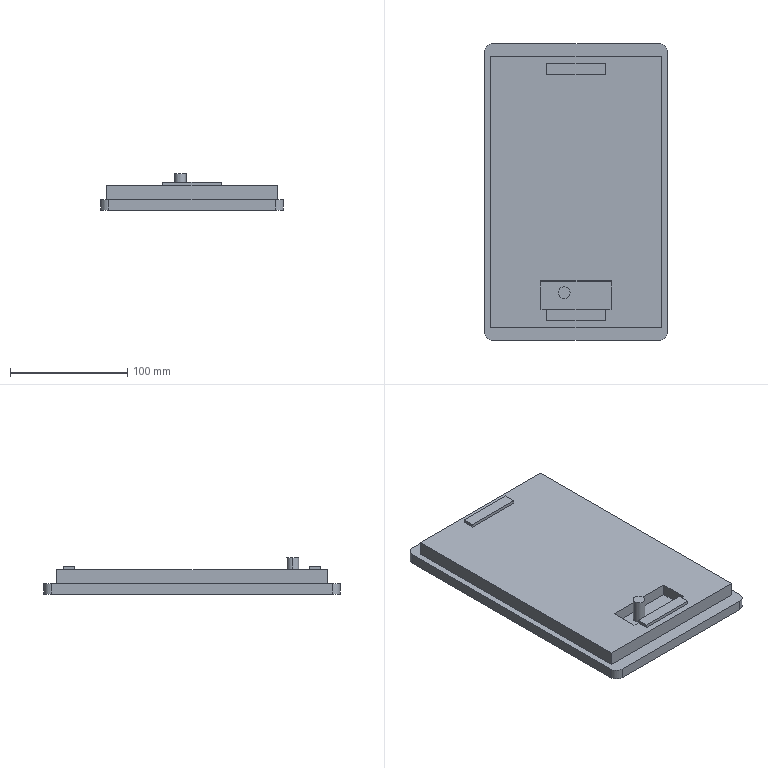Part | 1 solid | 37 faces | box 156 x 253.2 x 31 mm | volume 746157 mm3 | plane 31 | cylinder 6 | commonest cylinder face diameters 14 x4 10 x2
STEP:
#1=CARTESIAN_POINT('',(-5.,-86.,31.));
#2=VERTEX_POINT('',#1);
#3=CARTESIAN_POINT('',(-15.,-86.,31.));
#4=VERTEX_POINT('',#3);
#5=CARTESIAN_POINT('',(-10.,-86.,31.));
#6=DIRECTION('',(0.,0.,1.));
#7=DIRECTION('',(1.,0.,0.));
#8=AXIS2_PLACEMENT_3D('',#5,#6,#7);
#9=CIRCLE('',#8,5.);
#10=EDGE_CURVE('',#2,#4,#9,.T.);
#11=ORIENTED_EDGE('',*,*,#10,.F.);
#12=CARTESIAN_POINT('',(-5.,-86.,11.));
#13=VERTEX_POINT('',#12);
#14=CARTESIAN_POINT('',(-5.,-86.,31.));
#15=DIRECTION('',(0.,0.,-1.));
#16=VECTOR('',#15,1000.);
#17=LINE('',#14,#16);
#18=EDGE_CURVE('',#2,#13,#17,.T.);
#19=ORIENTED_EDGE('',*,*,#18,.T.);
#20=CARTESIAN_POINT('',(-15.,-86.,11.));
#21=VERTEX_POINT('',#20);
#22=CARTESIAN_POINT('',(-10.,-86.,11.));
#23=DIRECTION('',(0.,0.,1.));
#24=DIRECTION('',(1.,0.,0.));
#25=AXIS2_PLACEMENT_3D('',#22,#23,#24);
#26=CIRCLE('',#25,5.);
#27=EDGE_CURVE('',#13,#21,#26,.T.);
#28=ORIENTED_EDGE('',*,*,#27,.T.);
#29=CARTESIAN_POINT('',(-15.,-86.,31.));
#30=DIRECTION('',(0.,0.,-1.));
#31=VECTOR('',#30,1000.);
#32=LINE('',#29,#31);
#33=EDGE_CURVE('',#4,#21,#32,.T.);
#34=ORIENTED_EDGE('',*,*,#33,.F.);
#35=EDGE_LOOP('',(#11,#19,#28,#34));
#36=FACE_OUTER_BOUND('',#35,.T.);
#37=CARTESIAN_POINT('',(-10.,-86.,31.));
#38=DIRECTION('',(0.,0.,-1.));
#39=DIRECTION('',(-1.,0.,0.));
#40=AXIS2_PLACEMENT_3D('',#37,#38,#39);
#41=CYLINDRICAL_SURFACE('',#40,5.);
#42=ADVANCED_FACE('',(#36),#41,.T.);
#43=CARTESIAN_POINT('',(25.,-100.,21.));
#44=VERTEX_POINT('',#43);
#45=CARTESIAN_POINT('',(30.,-100.,21.));
#46=VERTEX_POINT('',#45);
#47=CARTESIAN_POINT('',(-30.,-100.,21.));
#48=DIRECTION('',(1.,0.,0.));
#49=VECTOR('',#48,1000.);
#50=LINE('',#47,#49);
#51=EDGE_CURVE('',#44,#46,#50,.T.);
#52=ORIENTED_EDGE('',*,*,#51,.F.);
#53=CARTESIAN_POINT('',(25.,-110.,21.));
#54=VERTEX_POINT('',#53);
#55=CARTESIAN_POINT('',(25.,-110.,21.));
#56=DIRECTION('',(0.,1.,0.));
#57=VECTOR('',#56,1000.);
#58=LINE('',#55,#57);
#59=EDGE_CURVE('',#54,#44,#58,.T.);
#60=ORIENTED_EDGE('',*,*,#59,.F.);
#61=CARTESIAN_POINT('',(-25.,-110.,21.));
#62=VERTEX_POINT('',#61);
#63=CARTESIAN_POINT('',(-25.,-110.,21.));
#64=DIRECTION('',(1.,0.,0.));
#65=VECTOR('',#64,1000.);
#66=LINE('',#63,#65);
#67=EDGE_CURVE('',#62,#54,#66,.T.);
#68=ORIENTED_EDGE('',*,*,#67,.F.);
#69=CARTESIAN_POINT('',(-25.,-100.,21.));
#70=VERTEX_POINT('',#69);
#71=CARTESIAN_POINT('',(-25.,-110.,21.));
#72=DIRECTION('',(0.,-1.,0.));
#73=VECTOR('',#72,1000.);
#74=LINE('',#71,#73);
#75=EDGE_CURVE('',#70,#62,#74,.T.);
#76=ORIENTED_EDGE('',*,*,#75,.F.);
#77=CARTESIAN_POINT('',(-30.,-100.,21.));
#78=VERTEX_POINT('',#77);
#79=CARTESIAN_POINT('',(-30.,-100.,21.));
#80=DIRECTION('',(1.,0.,0.));
#81=VECTOR('',#80,1000.);
#82=LINE('',#79,#81);
#83=EDGE_CURVE('',#78,#70,#82,.T.);
#84=ORIENTED_EDGE('',*,*,#83,.F.);
#85=CARTESIAN_POINT('',(-30.,-76.,21.));
#86=VERTEX_POINT('',#85);
#87=CARTESIAN_POINT('',(-30.,-76.,21.));
#88=DIRECTION('',(0.,-1.,0.));
#89=VECTOR('',#88,1000.);
#90=LINE('',#87,#89);
#91=EDGE_CURVE('',#86,#78,#90,.T.);
#92=ORIENTED_EDGE('',*,*,#91,.F.);
#93=CARTESIAN_POINT('',(30.,-76.,21.));
#94=VERTEX_POINT('',#93);
#95=CARTESIAN_POINT('',(-30.,-76.,21.));
#96=DIRECTION('',(-1.,0.,0.));
#97=VECTOR('',#96,1000.);
#98=LINE('',#95,#97);
#99=EDGE_CURVE('',#94,#86,#98,.T.);
#100=ORIENTED_EDGE('',*,*,#99,.F.);
#101=CARTESIAN_POINT('',(30.,-76.,21.));
#102=DIRECTION('',(0.,1.,0.));
#103=VECTOR('',#102,1000.);
#104=LINE('',#101,#103);
#105=EDGE_CURVE('',#46,#94,#104,.T.);
#106=ORIENTED_EDGE('',*,*,#105,.F.);
#107=EDGE_LOOP('',(#52,#60,#68,#76,#84,#92,#100,#106));
#108=FACE_BOUND('',#107,.T.);
#109=CARTESIAN_POINT('',(72.75,-115.5,21.));
#110=VERTEX_POINT('',#109);
#111=CARTESIAN_POINT('',(72.75,115.5,21.));
#112=VERTEX_POINT('',#111);
#113=CARTESIAN_POINT('',(72.75,115.5,21.));
#114=DIRECTION('',(0.,1.,0.));
#115=VECTOR('',#114,1000.);
#116=LINE('',#113,#115);
#117=EDGE_CURVE('',#110,#112,#116,.T.);
#118=ORIENTED_EDGE('',*,*,#117,.T.);
#119=CARTESIAN_POINT('',(-72.75,115.5,21.));
#120=VERTEX_POINT('',#119);
#121=CARTESIAN_POINT('',(-72.75,115.5,21.));
#122=DIRECTION('',(-1.,0.,0.));
#123=VECTOR('',#122,1000.);
#124=LINE('',#121,#123);
#125=EDGE_CURVE('',#112,#120,#124,.T.);
#126=ORIENTED_EDGE('',*,*,#125,.T.);
#127=CARTESIAN_POINT('',(-72.75,-115.5,21.));
#128=VERTEX_POINT('',#127);
#129=CARTESIAN_POINT('',(-72.75,115.5,21.));
#130=DIRECTION('',(0.,-1.,0.));
#131=VECTOR('',#130,1000.);
#132=LINE('',#129,#131);
#133=EDGE_CURVE('',#120,#128,#132,.T.);
#134=ORIENTED_EDGE('',*,*,#133,.T.);
#135=CARTESIAN_POINT('',(-72.75,-115.5,21.));
#136=DIRECTION('',(1.,0.,0.));
#137=VECTOR('',#136,1000.);
#138=LINE('',#135,#137);
#139=EDGE_CURVE('',#128,#110,#138,.T.);
#140=ORIENTED_EDGE('',*,*,#139,.T.);
#141=EDGE_LOOP('',(#118,#126,#134,#140));
#142=FACE_OUTER_BOUND('',#141,.T.);
#143=CARTESIAN_POINT('',(25.,110.,21.));
#144=VERTEX_POINT('',#143);
#145=CARTESIAN_POINT('',(-25.,110.,21.));
#146=VERTEX_POINT('',#145);
#147=CARTESIAN_POINT('',(-25.,110.,21.));
#148=DIRECTION('',(-1.,0.,0.));
#149=VECTOR('',#148,1000.);
#150=LINE('',#147,#149);
#151=EDGE_CURVE('',#144,#146,#150,.T.);
#152=ORIENTED_EDGE('',*,*,#151,.F.);
#153=CARTESIAN_POINT('',(25.,100.,21.));
#154=VERTEX_POINT('',#153);
#155=CARTESIAN_POINT('',(25.,110.,21.));
#156=DIRECTION('',(0.,1.,0.));
#157=VECTOR('',#156,1000.);
#158=LINE('',#155,#157);
#159=EDGE_CURVE('',#154,#144,#158,.T.);
#160=ORIENTED_EDGE('',*,*,#159,.F.);
#161=CARTESIAN_POINT('',(-25.,100.,21.));
#162=VERTEX_POINT('',#161);
#163=CARTESIAN_POINT('',(-25.,100.,21.));
#164=DIRECTION('',(1.,0.,0.));
#165=VECTOR('',#164,1000.);
#166=LINE('',#163,#165);
#167=EDGE_CURVE('',#162,#154,#166,.T.);
#168=ORIENTED_EDGE('',*,*,#167,.F.);
#169=CARTESIAN_POINT('',(-25.,110.,21.));
#170=DIRECTION('',(0.,-1.,0.));
#171=VECTOR('',#170,1000.);
#172=LINE('',#169,#171);
#173=EDGE_CURVE('',#146,#162,#172,.T.);
#174=ORIENTED_EDGE('',*,*,#173,.F.);
#175=EDGE_LOOP('',(#152,#160,#168,#174));
#176=FACE_BOUND('',#175,.T.);
#177=CARTESIAN_POINT('',(0.,0.,21.));
#178=DIRECTION('',(0.,0.,1.));
#179=DIRECTION('',(1.,0.,0.));
#180=AXIS2_PLACEMENT_3D('',#177,#178,#179);
#181=PLANE('',#180);
#182=ADVANCED_FACE('',(#108,#142,#176),#181,.T.);
#183=CARTESIAN_POINT('',(78.,-119.6,9.));
#184=VERTEX_POINT('',#183);
#185=CARTESIAN_POINT('',(78.,119.6,9.));
#186=VERTEX_POINT('',#185);
#187=CARTESIAN_POINT('',(78.,126.6,9.));
#188=DIRECTION('',(0.,1.,0.));
#189=VECTOR('',#188,1000.);
#190=LINE('',#187,#189);
#191=EDGE_CURVE('',#184,#186,#190,.T.);
#192=ORIENTED_EDGE('',*,*,#191,.F.);
#193=CARTESIAN_POINT('',(78.,-119.6,0.));
#194=VERTEX_POINT('',#193);
#195=CARTESIAN_POINT('',(78.,-119.6,9.));
#196=DIRECTION('',(0.,0.,-1.));
#197=VECTOR('',#196,1000.);
#198=LINE('',#195,#197);
#199=EDGE_CURVE('',#184,#194,#198,.T.);
#200=ORIENTED_EDGE('',*,*,#199,.T.);
#201=CARTESIAN_POINT('',(78.,119.6,0.));
#202=VERTEX_POINT('',#201);
#203=CARTESIAN_POINT('',(78.,126.6,0.));
#204=DIRECTION('',(0.,1.,0.));
#205=VECTOR('',#204,1000.);
#206=LINE('',#203,#205);
#207=EDGE_CURVE('',#194,#202,#206,.T.);
#208=ORIENTED_EDGE('',*,*,#207,.T.);
#209=CARTESIAN_POINT('',(78.,119.6,9.));
#210=DIRECTION('',(0.,0.,1.));
#211=VECTOR('',#210,1000.);
#212=LINE('',#209,#211);
#213=EDGE_CURVE('',#202,#186,#212,.T.);
#214=ORIENTED_EDGE('',*,*,#213,.T.);
#215=EDGE_LOOP('',(#192,#200,#208,#214));
#216=FACE_OUTER_BOUND('',#215,.T.);
#217=CARTESIAN_POINT('',(78.,126.6,9.));
#218=DIRECTION('',(-1.,0.,0.));
#219=DIRECTION('',(0.,-1.,0.));
#220=AXIS2_PLACEMENT_3D('',#217,#218,#219);
#221=PLANE('',#220);
#222=ADVANCED_FACE('',(#216),#221,.F.);
#223=CARTESIAN_POINT('',(71.,126.6,9.));
#224=VERTEX_POINT('',#223);
#225=CARTESIAN_POINT('',(-71.,126.6,9.));
#226=VERTEX_POINT('',#225);
#227=CARTESIAN_POINT('',(-78.,126.6,9.));
#228=DIRECTION('',(-1.,0.,0.));
#229=VECTOR('',#228,1000.);
#230=LINE('',#227,#229);
#231=EDGE_CURVE('',#224,#226,#230,.T.);
#232=ORIENTED_EDGE('',*,*,#231,.F.);
#233=CARTESIAN_POINT('',(71.,126.6,0.));
#234=VERTEX_POINT('',#233);
#235=CARTESIAN_POINT('',(71.,126.6,9.));
#236=DIRECTION('',(0.,0.,-1.));
#237=VECTOR('',#236,1000.);
#238=LINE('',#235,#237);
#239=EDGE_CURVE('',#224,#234,#238,.T.);
#240=ORIENTED_EDGE('',*,*,#239,.T.);
#241=CARTESIAN_POINT('',(-71.,126.6,0.));
#242=VERTEX_POINT('',#241);
#243=CARTESIAN_POINT('',(-78.,126.6,0.));
#244=DIRECTION('',(-1.,0.,0.));
#245=VECTOR('',#244,1000.);
#246=LINE('',#243,#245);
#247=EDGE_CURVE('',#234,#242,#246,.T.);
#248=ORIENTED_EDGE('',*,*,#247,.T.);
#249=CARTESIAN_POINT('',(-71.,126.6,9.));
#250=DIRECTION('',(0.,0.,1.));
#251=VECTOR('',#250,1000.);
#252=LINE('',#249,#251);
#253=EDGE_CURVE('',#242,#226,#252,.T.);
#254=ORIENTED_EDGE('',*,*,#253,.T.);
#255=EDGE_LOOP('',(#232,#240,#248,#254));
#256=FACE_OUTER_BOUND('',#255,.T.);
#257=CARTESIAN_POINT('',(-78.,126.6,9.));
#258=DIRECTION('',(0.,-1.,0.));
#259=DIRECTION('',(0.,0.,-1.));
#260=AXIS2_PLACEMENT_3D('',#257,#258,#259);
#261=PLANE('',#260);
#262=ADVANCED_FACE('',(#256),#261,.F.);
#263=CARTESIAN_POINT('',(-78.,119.6,0.));
#264=VERTEX_POINT('',#263);
#265=CARTESIAN_POINT('',(-78.,-119.6,0.));
#266=VERTEX_POINT('',#265);
#267=CARTESIAN_POINT('',(-78.,126.6,0.));
#268=DIRECTION('',(0.,-1.,0.));
#269=VECTOR('',#268,1000.);
#270=LINE('',#267,#269);
#271=EDGE_CURVE('',#264,#266,#270,.T.);
#272=ORIENTED_EDGE('',*,*,#271,.T.);
#273=CARTESIAN_POINT('',(-78.,-119.6,9.));
#274=VERTEX_POINT('',#273);
#275=CARTESIAN_POINT('',(-78.,-119.6,9.));
#276=DIRECTION('',(0.,0.,1.));
#277=VECTOR('',#276,1000.);
#278=LINE('',#275,#277);
#279=EDGE_CURVE('',#266,#274,#278,.T.);
#280=ORIENTED_EDGE('',*,*,#279,.T.);
#281=CARTESIAN_POINT('',(-78.,119.6,9.));
#282=VERTEX_POINT('',#281);
#283=CARTESIAN_POINT('',(-78.,126.6,9.));
#284=DIRECTION('',(0.,-1.,0.));
#285=VECTOR('',#284,1000.);
#286=LINE('',#283,#285);
#287=EDGE_CURVE('',#282,#274,#286,.T.);
#288=ORIENTED_EDGE('',*,*,#287,.F.);
#289=CARTESIAN_POINT('',(-78.,119.6,9.));
#290=DIRECTION('',(0.,0.,-1.));
#291=VECTOR('',#290,1000.);
#292=LINE('',#289,#291);
#293=EDGE_CURVE('',#282,#264,#292,.T.);
#294=ORIENTED_EDGE('',*,*,#293,.T.);
#295=EDGE_LOOP('',(#272,#280,#288,#294));
#296=FACE_OUTER_BOUND('',#295,.T.);
#297=CARTESIAN_POINT('',(-78.,126.6,9.));
#298=DIRECTION('',(1.,0.,0.));
#299=DIRECTION('',(0.,1.,0.));
#300=AXIS2_PLACEMENT_3D('',#297,#298,#299);
#301=PLANE('',#300);
#302=ADVANCED_FACE('',(#296),#301,.F.);
#303=CARTESIAN_POINT('',(-71.,-126.6,0.));
#304=VERTEX_POINT('',#303);
#305=CARTESIAN_POINT('',(71.,-126.6,0.));
#306=VERTEX_POINT('',#305);
#307=CARTESIAN_POINT('',(-78.,-126.6,0.));
#308=DIRECTION('',(1.,0.,0.));
#309=VECTOR('',#308,1000.);
#310=LINE('',#307,#309);
#311=EDGE_CURVE('',#304,#306,#310,.T.);
#312=ORIENTED_EDGE('',*,*,#311,.T.);
#313=CARTESIAN_POINT('',(71.,-126.6,9.));
#314=VERTEX_POINT('',#313);
#315=CARTESIAN_POINT('',(71.,-126.6,9.));
#316=DIRECTION('',(0.,0.,1.));
#317=VECTOR('',#316,1000.);
#318=LINE('',#315,#317);
#319=EDGE_CURVE('',#306,#314,#318,.T.);
#320=ORIENTED_EDGE('',*,*,#319,.T.);
#321=CARTESIAN_POINT('',(-71.,-126.6,9.));
#322=VERTEX_POINT('',#321);
#323=CARTESIAN_POINT('',(-78.,-126.6,9.));
#324=DIRECTION('',(1.,0.,0.));
#325=VECTOR('',#324,1000.);
#326=LINE('',#323,#325);
#327=EDGE_CURVE('',#322,#314,#326,.T.);
#328=ORIENTED_EDGE('',*,*,#327,.F.);
#329=CARTESIAN_POINT('',(-71.,-126.6,9.));
#330=DIRECTION('',(0.,0.,-1.));
#331=VECTOR('',#330,1000.);
#332=LINE('',#329,#331);
#333=EDGE_CURVE('',#322,#304,#332,.T.);
#334=ORIENTED_EDGE('',*,*,#333,.T.);
#335=EDGE_LOOP('',(#312,#320,#328,#334));
#336=FACE_OUTER_BOUND('',#335,.T.);
#337=CARTESIAN_POINT('',(-78.,-126.6,9.));
#338=DIRECTION('',(0.,1.,0.));
#339=DIRECTION('',(0.,0.,1.));
#340=AXIS2_PLACEMENT_3D('',#337,#338,#339);
#341=PLANE('',#340);
#342=ADVANCED_FACE('',(#336),#341,.F.);
#343=CARTESIAN_POINT('',(72.75,-115.5,9.));
#344=VERTEX_POINT('',#343);
#345=CARTESIAN_POINT('',(72.75,115.5,9.));
#346=VERTEX_POINT('',#345);
#347=CARTESIAN_POINT('',(72.75,115.5,9.));
#348=DIRECTION('',(0.,1.,0.));
#349=VECTOR('',#348,1000.);
#350=LINE('',#347,#349);
#351=EDGE_CURVE('',#344,#346,#350,.T.);
#352=ORIENTED_EDGE('',*,*,#351,.F.);
#353=CARTESIAN_POINT('',(-72.75,-115.5,9.));
#354=VERTEX_POINT('',#353);
#355=CARTESIAN_POINT('',(-72.75,-115.5,9.));
#356=DIRECTION('',(1.,0.,0.));
#357=VECTOR('',#356,1000.);
#358=LINE('',#355,#357);
#359=EDGE_CURVE('',#354,#344,#358,.T.);
#360=ORIENTED_EDGE('',*,*,#359,.F.);
#361=CARTESIAN_POINT('',(-72.75,115.5,9.));
#362=VERTEX_POINT('',#361);
#363=CARTESIAN_POINT('',(-72.75,115.5,9.));
#364=DIRECTION('',(0.,-1.,0.));
#365=VECTOR('',#364,1000.);
#366=LINE('',#363,#365);
#367=EDGE_CURVE('',#362,#354,#366,.T.);
#368=ORIENTED_EDGE('',*,*,#367,.F.);
#369=CARTESIAN_POINT('',(-72.75,115.5,9.));
#370=DIRECTION('',(-1.,0.,0.));
#371=VECTOR('',#370,1000.);
#372=LINE('',#369,#371);
#373=EDGE_CURVE('',#346,#362,#372,.T.);
#374=ORIENTED_EDGE('',*,*,#373,.F.);
#375=EDGE_LOOP('',(#352,#360,#368,#374));
#376=FACE_BOUND('',#375,.T.);
#377=ORIENTED_EDGE('',*,*,#327,.T.);
#378=CARTESIAN_POINT('',(71.,-119.6,9.));
#379=DIRECTION('',(0.,0.,1.));
#380=DIRECTION('',(1.,0.,0.));
#381=AXIS2_PLACEMENT_3D('',#378,#379,#380);
#382=CIRCLE('',#381,7.);
#383=EDGE_CURVE('',#314,#184,#382,.T.);
#384=ORIENTED_EDGE('',*,*,#383,.T.);
#385=ORIENTED_EDGE('',*,*,#191,.T.);
#386=CARTESIAN_POINT('',(71.,119.6,9.));
#387=DIRECTION('',(0.,0.,1.));
#388=DIRECTION('',(1.,0.,0.));
#389=AXIS2_PLACEMENT_3D('',#386,#387,#388);
#390=CIRCLE('',#389,7.);
#391=EDGE_CURVE('',#186,#224,#390,.T.);
#392=ORIENTED_EDGE('',*,*,#391,.T.);
#393=ORIENTED_EDGE('',*,*,#231,.T.);
#394=CARTESIAN_POINT('',(-71.,119.6,9.));
#395=DIRECTION('',(0.,0.,1.));
#396=DIRECTION('',(1.,0.,0.));
#397=AXIS2_PLACEMENT_3D('',#394,#395,#396);
#398=CIRCLE('',#397,7.);
#399=EDGE_CURVE('',#226,#282,#398,.T.);
#400=ORIENTED_EDGE('',*,*,#399,.T.);
#401=ORIENTED_EDGE('',*,*,#287,.T.);
#402=CARTESIAN_POINT('',(-71.,-119.6,9.));
#403=DIRECTION('',(0.,0.,1.));
#404=DIRECTION('',(1.,0.,0.));
#405=AXIS2_PLACEMENT_3D('',#402,#403,#404);
#406=CIRCLE('',#405,7.);
#407=EDGE_CURVE('',#274,#322,#406,.T.);
#408=ORIENTED_EDGE('',*,*,#407,.T.);
#409=EDGE_LOOP('',(#377,#384,#385,#392,#393,#400,#401,#408));
#410=FACE_OUTER_BOUND('',#409,.T.);
#411=CARTESIAN_POINT('',(0.,0.,9.));
#412=DIRECTION('',(0.,0.,1.));
#413=DIRECTION('',(1.,0.,0.));
#414=AXIS2_PLACEMENT_3D('',#411,#412,#413);
#415=PLANE('',#414);
#416=ADVANCED_FACE('',(#376,#410),#415,.T.);
#417=CARTESIAN_POINT('',(-53.,101.6,0.));
#418=VERTEX_POINT('',#417);
#419=CARTESIAN_POINT('',(53.,101.6,0.));
#420=VERTEX_POINT('',#419);
#421=CARTESIAN_POINT('',(53.,101.6,0.));
#422=DIRECTION('',(1.,0.,0.));
#423=VECTOR('',#422,1000.);
#424=LINE('',#421,#423);
#425=EDGE_CURVE('',#418,#420,#424,.T.);
#426=ORIENTED_EDGE('',*,*,#425,.F.);
#427=CARTESIAN_POINT('',(-53.,-101.6,0.));
#428=VERTEX_POINT('',#427);
#429=CARTESIAN_POINT('',(-53.,101.6,0.));
#430=DIRECTION('',(0.,1.,0.));
#431=VECTOR('',#430,1000.);
#432=LINE('',#429,#431);
#433=EDGE_CURVE('',#428,#418,#432,.T.);
#434=ORIENTED_EDGE('',*,*,#433,.F.);
#435=CARTESIAN_POINT('',(53.,-101.6,0.));
#436=VERTEX_POINT('',#435);
#437=CARTESIAN_POINT('',(53.,-101.6,0.));
#438=DIRECTION('',(-1.,0.,0.));
#439=VECTOR('',#438,1000.);
#440=LINE('',#437,#439);
#441=EDGE_CURVE('',#436,#428,#440,.T.);
#442=ORIENTED_EDGE('',*,*,#441,.F.);
#443=CARTESIAN_POINT('',(53.,101.6,0.));
#444=DIRECTION('',(0.,-1.,0.));
#445=VECTOR('',#444,1000.);
#446=LINE('',#443,#445);
#447=EDGE_CURVE('',#420,#436,#446,.T.);
#448=ORIENTED_EDGE('',*,*,#447,.F.);
#449=EDGE_LOOP('',(#426,#434,#442,#448));
#450=FACE_BOUND('',#449,.T.);
#451=ORIENTED_EDGE('',*,*,#207,.F.);
#452=CARTESIAN_POINT('',(71.,-119.6,0.));
#453=DIRECTION('',(0.,0.,-1.));
#454=DIRECTION('',(1.,0.,0.));
#455=AXIS2_PLACEMENT_3D('',#452,#453,#454);
#456=CIRCLE('',#455,7.);
#457=EDGE_CURVE('',#194,#306,#456,.T.);
#458=ORIENTED_EDGE('',*,*,#457,.T.);
#459=ORIENTED_EDGE('',*,*,#311,.F.);
#460=CARTESIAN_POINT('',(-71.,-119.6,0.));
#461=DIRECTION('',(0.,0.,-1.));
#462=DIRECTION('',(1.,0.,0.));
#463=AXIS2_PLACEMENT_3D('',#460,#461,#462);
#464=CIRCLE('',#463,7.);
#465=EDGE_CURVE('',#304,#266,#464,.T.);
#466=ORIENTED_EDGE('',*,*,#465,.T.);
#467=ORIENTED_EDGE('',*,*,#271,.F.);
#468=CARTESIAN_POINT('',(-71.,119.6,0.));
#469=DIRECTION('',(0.,0.,-1.));
#470=DIRECTION('',(1.,0.,0.));
#471=AXIS2_PLACEMENT_3D('',#468,#469,#470);
#472=CIRCLE('',#471,7.);
#473=EDGE_CURVE('',#264,#242,#472,.T.);
#474=ORIENTED_EDGE('',*,*,#473,.T.);
#475=ORIENTED_EDGE('',*,*,#247,.F.);
#476=CARTESIAN_POINT('',(71.,119.6,0.));
#477=DIRECTION('',(0.,0.,-1.));
#478=DIRECTION('',(1.,0.,0.));
#479=AXIS2_PLACEMENT_3D('',#476,#477,#478);
#480=CIRCLE('',#479,7.);
#481=EDGE_CURVE('',#234,#202,#480,.T.);
#482=ORIENTED_EDGE('',*,*,#481,.T.);
#483=EDGE_LOOP('',(#451,#458,#459,#466,#467,#474,#475,#482));
#484=FACE_OUTER_BOUND('',#483,.T.);
#485=CARTESIAN_POINT('',(0.,0.,0.));
#486=DIRECTION('',(0.,0.,1.));
#487=DIRECTION('',(1.,0.,0.));
#488=AXIS2_PLACEMENT_3D('',#485,#486,#487);
#489=PLANE('',#488);
#490=ADVANCED_FACE('',(#450,#484),#489,.F.);
#491=ORIENTED_EDGE('',*,*,#383,.F.);
#492=ORIENTED_EDGE('',*,*,#319,.F.);
#493=ORIENTED_EDGE('',*,*,#457,.F.);
#494=ORIENTED_EDGE('',*,*,#199,.F.);
#495=EDGE_LOOP('',(#491,#492,#493,#494));
#496=FACE_OUTER_BOUND('',#495,.T.);
#497=CARTESIAN_POINT('',(71.,-119.6,9.));
#498=DIRECTION('',(0.,0.,-1.));
#499=DIRECTION('',(-1.,0.,0.));
#500=AXIS2_PLACEMENT_3D('',#497,#498,#499);
#501=CYLINDRICAL_SURFACE('',#500,7.);
#502=ADVANCED_FACE('',(#496),#501,.T.);
#503=ORIENTED_EDGE('',*,*,#407,.F.);
#504=ORIENTED_EDGE('',*,*,#279,.F.);
#505=ORIENTED_EDGE('',*,*,#465,.F.);
#506=ORIENTED_EDGE('',*,*,#333,.F.);
#507=EDGE_LOOP('',(#503,#504,#505,#506));
#508=FACE_OUTER_BOUND('',#507,.T.);
#509=CARTESIAN_POINT('',(-71.,-119.6,9.));
#510=DIRECTION('',(0.,0.,-1.));
#511=DIRECTION('',(-1.,0.,0.));
#512=AXIS2_PLACEMENT_3D('',#509,#510,#511);
#513=CYLINDRICAL_SURFACE('',#512,7.);
#514=ADVANCED_FACE('',(#508),#513,.T.);
#515=ORIENTED_EDGE('',*,*,#391,.F.);
#516=ORIENTED_EDGE('',*,*,#213,.F.);
#517=ORIENTED_EDGE('',*,*,#481,.F.);
#518=ORIENTED_EDGE('',*,*,#239,.F.);
#519=EDGE_LOOP('',(#515,#516,#517,#518));
#520=FACE_OUTER_BOUND('',#519,.T.);
#521=CARTESIAN_POINT('',(71.,119.6,9.));
#522=DIRECTION('',(0.,0.,-1.));
#523=DIRECTION('',(-1.,0.,0.));
#524=AXIS2_PLACEMENT_3D('',#521,#522,#523);
#525=CYLINDRICAL_SURFACE('',#524,7.);
#526=ADVANCED_FACE('',(#520),#525,.T.);
#527=ORIENTED_EDGE('',*,*,#399,.F.);
#528=ORIENTED_EDGE('',*,*,#253,.F.);
#529=ORIENTED_EDGE('',*,*,#473,.F.);
#530=ORIENTED_EDGE('',*,*,#293,.F.);
#531=EDGE_LOOP('',(#527,#528,#529,#530));
#532=FACE_OUTER_BOUND('',#531,.T.);
#533=CARTESIAN_POINT('',(-71.,119.6,9.));
#534=DIRECTION('',(0.,0.,-1.));
#535=DIRECTION('',(-1.,0.,0.));
#536=AXIS2_PLACEMENT_3D('',#533,#534,#535);
#537=CYLINDRICAL_SURFACE('',#536,7.);
#538=ADVANCED_FACE('',(#532),#537,.T.);
#539=ORIENTED_EDGE('',*,*,#351,.T.);
#540=CARTESIAN_POINT('',(72.75,115.5,21.));
#541=DIRECTION('',(0.,0.,-1.));
#542=VECTOR('',#541,1000.);
#543=LINE('',#540,#542);
#544=EDGE_CURVE('',#112,#346,#543,.T.);
#545=ORIENTED_EDGE('',*,*,#544,.F.);
#546=ORIENTED_EDGE('',*,*,#117,.F.);
#547=CARTESIAN_POINT('',(72.75,-115.5,21.));
#548=DIRECTION('',(0.,0.,-1.));
#549=VECTOR('',#548,1000.);
#550=LINE('',#547,#549);
#551=EDGE_CURVE('',#110,#344,#550,.T.);
#552=ORIENTED_EDGE('',*,*,#551,.T.);
#553=EDGE_LOOP('',(#539,#545,#546,#552));
#554=FACE_OUTER_BOUND('',#553,.T.);
#555=CARTESIAN_POINT('',(72.75,115.5,21.));
#556=DIRECTION('',(-1.,0.,0.));
#557=DIRECTION('',(0.,-1.,0.));
#558=AXIS2_PLACEMENT_3D('',#555,#556,#557);
#559=PLANE('',#558);
#560=ADVANCED_FACE('',(#554),#559,.F.);
#561=ORIENTED_EDGE('',*,*,#373,.T.);
#562=CARTESIAN_POINT('',(-72.75,115.5,21.));
#563=DIRECTION('',(0.,0.,-1.));
#564=VECTOR('',#563,1000.);
#565=LINE('',#562,#564);
#566=EDGE_CURVE('',#120,#362,#565,.T.);
#567=ORIENTED_EDGE('',*,*,#566,.F.);
#568=ORIENTED_EDGE('',*,*,#125,.F.);
#569=ORIENTED_EDGE('',*,*,#544,.T.);
#570=EDGE_LOOP('',(#561,#567,#568,#569));
#571=FACE_OUTER_BOUND('',#570,.T.);
#572=CARTESIAN_POINT('',(-72.75,115.5,21.));
#573=DIRECTION('',(0.,-1.,0.));
#574=DIRECTION('',(0.,0.,-1.));
#575=AXIS2_PLACEMENT_3D('',#572,#573,#574);
#576=PLANE('',#575);
#577=ADVANCED_FACE('',(#571),#576,.F.);
#578=ORIENTED_EDGE('',*,*,#367,.T.);
#579=CARTESIAN_POINT('',(-72.75,-115.5,21.));
#580=DIRECTION('',(0.,0.,-1.));
#581=VECTOR('',#580,1000.);
#582=LINE('',#579,#581);
#583=EDGE_CURVE('',#128,#354,#582,.T.);
#584=ORIENTED_EDGE('',*,*,#583,.F.);
#585=ORIENTED_EDGE('',*,*,#133,.F.);
#586=ORIENTED_EDGE('',*,*,#566,.T.);
#587=EDGE_LOOP('',(#578,#584,#585,#586));
#588=FACE_OUTER_BOUND('',#587,.T.);
#589=CARTESIAN_POINT('',(-72.75,115.5,21.));
#590=DIRECTION('',(1.,0.,0.));
#591=DIRECTION('',(0.,1.,0.));
#592=AXIS2_PLACEMENT_3D('',#589,#590,#591);
#593=PLANE('',#592);
#594=ADVANCED_FACE('',(#588),#593,.F.);
#595=ORIENTED_EDGE('',*,*,#359,.T.);
#596=ORIENTED_EDGE('',*,*,#551,.F.);
#597=ORIENTED_EDGE('',*,*,#139,.F.);
#598=ORIENTED_EDGE('',*,*,#583,.T.);
#599=EDGE_LOOP('',(#595,#596,#597,#598));
#600=FACE_OUTER_BOUND('',#599,.T.);
#601=CARTESIAN_POINT('',(-72.75,-115.5,21.));
#602=DIRECTION('',(0.,1.,0.));
#603=DIRECTION('',(0.,0.,1.));
#604=AXIS2_PLACEMENT_3D('',#601,#602,#603);
#605=PLANE('',#604);
#606=ADVANCED_FACE('',(#600),#605,.F.);
#607=ORIENTED_EDGE('',*,*,#433,.T.);
#608=CARTESIAN_POINT('',(-53.,101.6,0.1));
#609=VERTEX_POINT('',#608);
#610=CARTESIAN_POINT('',(-53.,101.6,0.1));
#611=DIRECTION('',(0.,0.,-1.));
#612=VECTOR('',#611,1000.);
#613=LINE('',#610,#612);
#614=EDGE_CURVE('',#609,#418,#613,.T.);
#615=ORIENTED_EDGE('',*,*,#614,.F.);
#616=CARTESIAN_POINT('',(-53.,-101.6,0.1));
#617=VERTEX_POINT('',#616);
#618=CARTESIAN_POINT('',(-53.,101.6,0.1));
#619=DIRECTION('',(0.,1.,0.));
#620=VECTOR('',#619,1000.);
#621=LINE('',#618,#620);
#622=EDGE_CURVE('',#617,#609,#621,.T.);
#623=ORIENTED_EDGE('',*,*,#622,.F.);
#624=CARTESIAN_POINT('',(-53.,-101.6,0.1));
#625=DIRECTION('',(0.,0.,-1.));
#626=VECTOR('',#625,1000.);
#627=LINE('',#624,#626);
#628=EDGE_CURVE('',#617,#428,#627,.T.);
#629=ORIENTED_EDGE('',*,*,#628,.T.);
#630=EDGE_LOOP('',(#607,#615,#623,#629));
#631=FACE_OUTER_BOUND('',#630,.T.);
#632=CARTESIAN_POINT('',(-53.,101.6,0.1));
#633=DIRECTION('',(-1.,0.,0.));
#634=DIRECTION('',(0.,0.,1.));
#635=AXIS2_PLACEMENT_3D('',#632,#633,#634);
#636=PLANE('',#635);
#637=ADVANCED_FACE('',(#631),#636,.F.);
#638=ORIENTED_EDGE('',*,*,#441,.T.);
#639=ORIENTED_EDGE('',*,*,#628,.F.);
#640=CARTESIAN_POINT('',(53.,-101.6,0.1));
#641=VERTEX_POINT('',#640);
#642=CARTESIAN_POINT('',(53.,-101.6,0.1));
#643=DIRECTION('',(-1.,0.,0.));
#644=VECTOR('',#643,1000.);
#645=LINE('',#642,#644);
#646=EDGE_CURVE('',#641,#617,#645,.T.);
#647=ORIENTED_EDGE('',*,*,#646,.F.);
#648=CARTESIAN_POINT('',(53.,-101.6,0.1));
#649=DIRECTION('',(0.,0.,-1.));
#650=VECTOR('',#649,1000.);
#651=LINE('',#648,#650);
#652=EDGE_CURVE('',#641,#436,#651,.T.);
#653=ORIENTED_EDGE('',*,*,#652,.T.);
#654=EDGE_LOOP('',(#638,#639,#647,#653));
#655=FACE_OUTER_BOUND('',#654,.T.);
#656=CARTESIAN_POINT('',(53.,-101.6,0.1));
#657=DIRECTION('',(0.,-1.,0.));
#658=DIRECTION('',(0.,0.,-1.));
#659=AXIS2_PLACEMENT_3D('',#656,#657,#658);
#660=PLANE('',#659);
#661=ADVANCED_FACE('',(#655),#660,.F.);
#662=ORIENTED_EDGE('',*,*,#447,.T.);
#663=ORIENTED_EDGE('',*,*,#652,.F.);
#664=CARTESIAN_POINT('',(53.,101.6,0.1));
#665=VERTEX_POINT('',#664);
#666=CARTESIAN_POINT('',(53.,101.6,0.1));
#667=DIRECTION('',(0.,-1.,0.));
#668=VECTOR('',#667,1000.);
#669=LINE('',#666,#668);
#670=EDGE_CURVE('',#665,#641,#669,.T.);
#671=ORIENTED_EDGE('',*,*,#670,.F.);
#672=CARTESIAN_POINT('',(53.,101.6,0.1));
#673=DIRECTION('',(0.,0.,-1.));
#674=VECTOR('',#673,1000.);
#675=LINE('',#672,#674);
#676=EDGE_CURVE('',#665,#420,#675,.T.);
#677=ORIENTED_EDGE('',*,*,#676,.T.);
#678=EDGE_LOOP('',(#662,#663,#671,#677));
#679=FACE_OUTER_BOUND('',#678,.T.);
#680=CARTESIAN_POINT('',(53.,101.6,0.1));
#681=DIRECTION('',(1.,0.,0.));
#682=DIRECTION('',(0.,0.,-1.));
#683=AXIS2_PLACEMENT_3D('',#680,#681,#682);
#684=PLANE('',#683);
#685=ADVANCED_FACE('',(#679),#684,.F.);
#686=ORIENTED_EDGE('',*,*,#425,.T.);
#687=ORIENTED_EDGE('',*,*,#676,.F.);
#688=CARTESIAN_POINT('',(53.,101.6,0.1));
#689=DIRECTION('',(1.,0.,0.));
#690=VECTOR('',#689,1000.);
#691=LINE('',#688,#690);
#692=EDGE_CURVE('',#609,#665,#691,.T.);
#693=ORIENTED_EDGE('',*,*,#692,.F.);
#694=ORIENTED_EDGE('',*,*,#614,.T.);
#695=EDGE_LOOP('',(#686,#687,#693,#694));
#696=FACE_OUTER_BOUND('',#695,.T.);
#697=CARTESIAN_POINT('',(53.,101.6,0.1));
#698=DIRECTION('',(0.,1.,0.));
#699=DIRECTION('',(0.,0.,1.));
#700=AXIS2_PLACEMENT_3D('',#697,#698,#699);
#701=PLANE('',#700);
#702=ADVANCED_FACE('',(#696),#701,.F.);
#703=ORIENTED_EDGE('',*,*,#622,.T.);
#704=ORIENTED_EDGE('',*,*,#692,.T.);
#705=ORIENTED_EDGE('',*,*,#670,.T.);
#706=ORIENTED_EDGE('',*,*,#646,.T.);
#707=EDGE_LOOP('',(#703,#704,#705,#706));
#708=FACE_OUTER_BOUND('',#707,.T.);
#709=CARTESIAN_POINT('',(0.,0.,0.1));
#710=DIRECTION('',(0.,0.,-1.));
#711=DIRECTION('',(-1.,0.,0.));
#712=AXIS2_PLACEMENT_3D('',#709,#710,#711);
#713=PLANE('',#712);
#714=ADVANCED_FACE('',(#708),#713,.T.);
#715=ORIENTED_EDGE('',*,*,#159,.T.);
#716=CARTESIAN_POINT('',(25.,110.,23.7));
#717=VERTEX_POINT('',#716);
#718=CARTESIAN_POINT('',(25.,110.,23.7));
#719=DIRECTION('',(0.,0.,-1.));
#720=VECTOR('',#719,1000.);
#721=LINE('',#718,#720);
#722=EDGE_CURVE('',#717,#144,#721,.T.);
#723=ORIENTED_EDGE('',*,*,#722,.F.);
#724=CARTESIAN_POINT('',(25.,100.,23.7));
#725=VERTEX_POINT('',#724);
#726=CARTESIAN_POINT('',(25.,110.,23.7));
#727=DIRECTION('',(0.,1.,0.));
#728=VECTOR('',#727,1000.);
#729=LINE('',#726,#728);
#730=EDGE_CURVE('',#725,#717,#729,.T.);
#731=ORIENTED_EDGE('',*,*,#730,.F.);
#732=CARTESIAN_POINT('',(25.,100.,23.7));
#733=DIRECTION('',(0.,0.,-1.));
#734=VECTOR('',#733,1000.);
#735=LINE('',#732,#734);
#736=EDGE_CURVE('',#725,#154,#735,.T.);
#737=ORIENTED_EDGE('',*,*,#736,.T.);
#738=EDGE_LOOP('',(#715,#723,#731,#737));
#739=FACE_OUTER_BOUND('',#738,.T.);
#740=CARTESIAN_POINT('',(25.,110.,23.7));
#741=DIRECTION('',(-1.,0.,0.));
#742=DIRECTION('',(0.,0.,1.));
#743=AXIS2_PLACEMENT_3D('',#740,#741,#742);
#744=PLANE('',#743);
#745=ADVANCED_FACE('',(#739),#744,.F.);
#746=ORIENTED_EDGE('',*,*,#151,.T.);
#747=CARTESIAN_POINT('',(-25.,110.,23.7));
#748=VERTEX_POINT('',#747);
#749=CARTESIAN_POINT('',(-25.,110.,23.7));
#750=DIRECTION('',(0.,0.,-1.));
#751=VECTOR('',#750,1000.);
#752=LINE('',#749,#751);
#753=EDGE_CURVE('',#748,#146,#752,.T.);
#754=ORIENTED_EDGE('',*,*,#753,.F.);
#755=CARTESIAN_POINT('',(-25.,110.,23.7));
#756=DIRECTION('',(-1.,0.,0.));
#757=VECTOR('',#756,1000.);
#758=LINE('',#755,#757);
#759=EDGE_CURVE('',#717,#748,#758,.T.);
#760=ORIENTED_EDGE('',*,*,#759,.F.);
#761=ORIENTED_EDGE('',*,*,#722,.T.);
#762=EDGE_LOOP('',(#746,#754,#760,#761));
#763=FACE_OUTER_BOUND('',#762,.T.);
#764=CARTESIAN_POINT('',(-25.,110.,23.7));
#765=DIRECTION('',(0.,-1.,0.));
#766=DIRECTION('',(0.,0.,-1.));
#767=AXIS2_PLACEMENT_3D('',#764,#765,#766);
#768=PLANE('',#767);
#769=ADVANCED_FACE('',(#763),#768,.F.);
#770=ORIENTED_EDGE('',*,*,#173,.T.);
#771=CARTESIAN_POINT('',(-25.,100.,23.7));
#772=VERTEX_POINT('',#771);
#773=CARTESIAN_POINT('',(-25.,100.,23.7));
#774=DIRECTION('',(0.,0.,-1.));
#775=VECTOR('',#774,1000.);
#776=LINE('',#773,#775);
#777=EDGE_CURVE('',#772,#162,#776,.T.);
#778=ORIENTED_EDGE('',*,*,#777,.F.);
#779=CARTESIAN_POINT('',(-25.,110.,23.7));
#780=DIRECTION('',(0.,-1.,0.));
#781=VECTOR('',#780,1000.);
#782=LINE('',#779,#781);
#783=EDGE_CURVE('',#748,#772,#782,.T.);
#784=ORIENTED_EDGE('',*,*,#783,.F.);
#785=ORIENTED_EDGE('',*,*,#753,.T.);
#786=EDGE_LOOP('',(#770,#778,#784,#785));
#787=FACE_OUTER_BOUND('',#786,.T.);
#788=CARTESIAN_POINT('',(-25.,110.,23.7));
#789=DIRECTION('',(1.,0.,0.));
#790=DIRECTION('',(0.,0.,-1.));
#791=AXIS2_PLACEMENT_3D('',#788,#789,#790);
#792=PLANE('',#791);
#793=ADVANCED_FACE('',(#787),#792,.F.);
#794=ORIENTED_EDGE('',*,*,#167,.T.);
#795=ORIENTED_EDGE('',*,*,#736,.F.);
#796=CARTESIAN_POINT('',(-25.,100.,23.7));
#797=DIRECTION('',(1.,0.,0.));
#798=VECTOR('',#797,1000.);
#799=LINE('',#796,#798);
#800=EDGE_CURVE('',#772,#725,#799,.T.);
#801=ORIENTED_EDGE('',*,*,#800,.F.);
#802=ORIENTED_EDGE('',*,*,#777,.T.);
#803=EDGE_LOOP('',(#794,#795,#801,#802));
#804=FACE_OUTER_BOUND('',#803,.T.);
#805=CARTESIAN_POINT('',(-25.,100.,23.7));
#806=DIRECTION('',(0.,1.,0.));
#807=DIRECTION('',(0.,0.,1.));
#808=AXIS2_PLACEMENT_3D('',#805,#806,#807);
#809=PLANE('',#808);
#810=ADVANCED_FACE('',(#804),#809,.F.);
#811=ORIENTED_EDGE('',*,*,#730,.T.);
#812=ORIENTED_EDGE('',*,*,#759,.T.);
#813=ORIENTED_EDGE('',*,*,#783,.T.);
#814=ORIENTED_EDGE('',*,*,#800,.T.);
#815=EDGE_LOOP('',(#811,#812,#813,#814));
#816=FACE_OUTER_BOUND('',#815,.T.);
#817=CARTESIAN_POINT('',(0.,0.,23.7));
#818=DIRECTION('',(0.,0.,1.));
#819=DIRECTION('',(1.,0.,0.));
#820=AXIS2_PLACEMENT_3D('',#817,#818,#819);
#821=PLANE('',#820);
#822=ADVANCED_FACE('',(#816),#821,.T.);
#823=ORIENTED_EDGE('',*,*,#75,.T.);
#824=CARTESIAN_POINT('',(-25.,-110.,23.7));
#825=VERTEX_POINT('',#824);
#826=CARTESIAN_POINT('',(-25.,-110.,23.7));
#827=DIRECTION('',(0.,0.,-1.));
#828=VECTOR('',#827,1000.);
#829=LINE('',#826,#828);
#830=EDGE_CURVE('',#825,#62,#829,.T.);
#831=ORIENTED_EDGE('',*,*,#830,.F.);
#832=CARTESIAN_POINT('',(-25.,-100.,23.7));
#833=VERTEX_POINT('',#832);
#834=CARTESIAN_POINT('',(-25.,-110.,23.7));
#835=DIRECTION('',(0.,-1.,0.));
#836=VECTOR('',#835,1000.);
#837=LINE('',#834,#836);
#838=EDGE_CURVE('',#833,#825,#837,.T.);
#839=ORIENTED_EDGE('',*,*,#838,.F.);
#840=CARTESIAN_POINT('',(-25.,-100.,23.7));
#841=DIRECTION('',(0.,0.,-1.));
#842=VECTOR('',#841,1000.);
#843=LINE('',#840,#842);
#844=EDGE_CURVE('',#833,#70,#843,.T.);
#845=ORIENTED_EDGE('',*,*,#844,.T.);
#846=EDGE_LOOP('',(#823,#831,#839,#845));
#847=FACE_OUTER_BOUND('',#846,.T.);
#848=CARTESIAN_POINT('',(-25.,-110.,23.7));
#849=DIRECTION('',(1.,0.,0.));
#850=DIRECTION('',(0.,0.,-1.));
#851=AXIS2_PLACEMENT_3D('',#848,#849,#850);
#852=PLANE('',#851);
#853=ADVANCED_FACE('',(#847),#852,.F.);
#854=ORIENTED_EDGE('',*,*,#67,.T.);
#855=CARTESIAN_POINT('',(25.,-110.,23.7));
#856=VERTEX_POINT('',#855);
#857=CARTESIAN_POINT('',(25.,-110.,23.7));
#858=DIRECTION('',(0.,0.,-1.));
#859=VECTOR('',#858,1000.);
#860=LINE('',#857,#859);
#861=EDGE_CURVE('',#856,#54,#860,.T.);
#862=ORIENTED_EDGE('',*,*,#861,.F.);
#863=CARTESIAN_POINT('',(-25.,-110.,23.7));
#864=DIRECTION('',(1.,0.,0.));
#865=VECTOR('',#864,1000.);
#866=LINE('',#863,#865);
#867=EDGE_CURVE('',#825,#856,#866,.T.);
#868=ORIENTED_EDGE('',*,*,#867,.F.);
#869=ORIENTED_EDGE('',*,*,#830,.T.);
#870=EDGE_LOOP('',(#854,#862,#868,#869));
#871=FACE_OUTER_BOUND('',#870,.T.);
#872=CARTESIAN_POINT('',(-25.,-110.,23.7));
#873=DIRECTION('',(0.,1.,0.));
#874=DIRECTION('',(0.,0.,1.));
#875=AXIS2_PLACEMENT_3D('',#872,#873,#874);
#876=PLANE('',#875);
#877=ADVANCED_FACE('',(#871),#876,.F.);
#878=ORIENTED_EDGE('',*,*,#59,.T.);
#879=CARTESIAN_POINT('',(25.,-100.,23.7));
#880=VERTEX_POINT('',#879);
#881=CARTESIAN_POINT('',(25.,-100.,23.7));
#882=DIRECTION('',(0.,0.,-1.));
#883=VECTOR('',#882,1000.);
#884=LINE('',#881,#883);
#885=EDGE_CURVE('',#880,#44,#884,.T.);
#886=ORIENTED_EDGE('',*,*,#885,.F.);
#887=CARTESIAN_POINT('',(25.,-110.,23.7));
#888=DIRECTION('',(0.,1.,0.));
#889=VECTOR('',#888,1000.);
#890=LINE('',#887,#889);
#891=EDGE_CURVE('',#856,#880,#890,.T.);
#892=ORIENTED_EDGE('',*,*,#891,.F.);
#893=ORIENTED_EDGE('',*,*,#861,.T.);
#894=EDGE_LOOP('',(#878,#886,#892,#893));
#895=FACE_OUTER_BOUND('',#894,.T.);
#896=CARTESIAN_POINT('',(25.,-110.,23.7));
#897=DIRECTION('',(-1.,0.,0.));
#898=DIRECTION('',(0.,0.,1.));
#899=AXIS2_PLACEMENT_3D('',#896,#897,#898);
#900=PLANE('',#899);
#901=ADVANCED_FACE('',(#895),#900,.F.);
#902=ORIENTED_EDGE('',*,*,#885,.T.);
#903=ORIENTED_EDGE('',*,*,#51,.T.);
#904=CARTESIAN_POINT('',(30.,-100.,11.));
#905=VERTEX_POINT('',#904);
#906=CARTESIAN_POINT('',(30.,-100.,11.));
#907=DIRECTION('',(0.,0.,1.));
#908=VECTOR('',#907,1000.);
#909=LINE('',#906,#908);
#910=EDGE_CURVE('',#905,#46,#909,.T.);
#911=ORIENTED_EDGE('',*,*,#910,.F.);
#912=CARTESIAN_POINT('',(-30.,-100.,11.));
#913=VERTEX_POINT('',#912);
#914=CARTESIAN_POINT('',(-30.,-100.,11.));
#915=DIRECTION('',(1.,0.,0.));
#916=VECTOR('',#915,1000.);
#917=LINE('',#914,#916);
#918=EDGE_CURVE('',#913,#905,#917,.T.);
#919=ORIENTED_EDGE('',*,*,#918,.F.);
#920=CARTESIAN_POINT('',(-30.,-100.,11.));
#921=DIRECTION('',(0.,0.,1.));
#922=VECTOR('',#921,1000.);
#923=LINE('',#920,#922);
#924=EDGE_CURVE('',#913,#78,#923,.T.);
#925=ORIENTED_EDGE('',*,*,#924,.T.);
#926=ORIENTED_EDGE('',*,*,#83,.T.);
#927=ORIENTED_EDGE('',*,*,#844,.F.);
#928=CARTESIAN_POINT('',(-25.,-100.,23.7));
#929=DIRECTION('',(-1.,0.,0.));
#930=VECTOR('',#929,1000.);
#931=LINE('',#928,#930);
#932=EDGE_CURVE('',#880,#833,#931,.T.);
#933=ORIENTED_EDGE('',*,*,#932,.F.);
#934=EDGE_LOOP('',(#902,#903,#911,#919,#925,#926,#927,#933));
#935=FACE_OUTER_BOUND('',#934,.T.);
#936=CARTESIAN_POINT('',(-25.,-100.,23.7));
#937=DIRECTION('',(0.,-1.,0.));
#938=DIRECTION('',(0.,0.,-1.));
#939=AXIS2_PLACEMENT_3D('',#936,#937,#938);
#940=PLANE('',#939);
#941=ADVANCED_FACE('',(#935),#940,.F.);
#942=ORIENTED_EDGE('',*,*,#838,.T.);
#943=ORIENTED_EDGE('',*,*,#867,.T.);
#944=ORIENTED_EDGE('',*,*,#891,.T.);
#945=ORIENTED_EDGE('',*,*,#932,.T.);
#946=EDGE_LOOP('',(#942,#943,#944,#945));
#947=FACE_OUTER_BOUND('',#946,.T.);
#948=CARTESIAN_POINT('',(0.,0.,23.7));
#949=DIRECTION('',(0.,0.,-1.));
#950=DIRECTION('',(-1.,0.,0.));
#951=AXIS2_PLACEMENT_3D('',#948,#949,#950);
#952=PLANE('',#951);
#953=ADVANCED_FACE('',(#947),#952,.F.);
#954=ORIENTED_EDGE('',*,*,#105,.T.);
#955=CARTESIAN_POINT('',(30.,-76.,11.));
#956=VERTEX_POINT('',#955);
#957=CARTESIAN_POINT('',(30.,-76.,11.));
#958=DIRECTION('',(0.,0.,1.));
#959=VECTOR('',#958,1000.);
#960=LINE('',#957,#959);
#961=EDGE_CURVE('',#956,#94,#960,.T.);
#962=ORIENTED_EDGE('',*,*,#961,.F.);
#963=CARTESIAN_POINT('',(30.,-76.,11.));
#964=DIRECTION('',(0.,1.,0.));
#965=VECTOR('',#964,1000.);
#966=LINE('',#963,#965);
#967=EDGE_CURVE('',#905,#956,#966,.T.);
#968=ORIENTED_EDGE('',*,*,#967,.F.);
#969=ORIENTED_EDGE('',*,*,#910,.T.);
#970=EDGE_LOOP('',(#954,#962,#968,#969));
#971=FACE_OUTER_BOUND('',#970,.T.);
#972=CARTESIAN_POINT('',(30.,-76.,11.));
#973=DIRECTION('',(1.,0.,0.));
#974=DIRECTION('',(0.,1.,0.));
#975=AXIS2_PLACEMENT_3D('',#972,#973,#974);
#976=PLANE('',#975);
#977=ADVANCED_FACE('',(#971),#976,.F.);
#978=ORIENTED_EDGE('',*,*,#91,.T.);
#979=ORIENTED_EDGE('',*,*,#924,.F.);
#980=CARTESIAN_POINT('',(-30.,-76.,11.));
#981=VERTEX_POINT('',#980);
#982=CARTESIAN_POINT('',(-30.,-76.,11.));
#983=DIRECTION('',(0.,-1.,0.));
#984=VECTOR('',#983,1000.);
#985=LINE('',#982,#984);
#986=EDGE_CURVE('',#981,#913,#985,.T.);
#987=ORIENTED_EDGE('',*,*,#986,.F.);
#988=CARTESIAN_POINT('',(-30.,-76.,11.));
#989=DIRECTION('',(0.,0.,1.));
#990=VECTOR('',#989,1000.);
#991=LINE('',#988,#990);
#992=EDGE_CURVE('',#981,#86,#991,.T.);
#993=ORIENTED_EDGE('',*,*,#992,.T.);
#994=EDGE_LOOP('',(#978,#979,#987,#993));
#995=FACE_OUTER_BOUND('',#994,.T.);
#996=CARTESIAN_POINT('',(-30.,-76.,11.));
#997=DIRECTION('',(-1.,0.,0.));
#998=DIRECTION('',(0.,-1.,0.));
#999=AXIS2_PLACEMENT_3D('',#996,#997,#998);
#1000=PLANE('',#999);
#1001=ADVANCED_FACE('',(#995),#1000,.F.);
#1002=ORIENTED_EDGE('',*,*,#99,.T.);
#1003=ORIENTED_EDGE('',*,*,#992,.F.);
#1004=CARTESIAN_POINT('',(-30.,-76.,11.));
#1005=DIRECTION('',(-1.,0.,0.));
#1006=VECTOR('',#1005,1000.);
#1007=LINE('',#1004,#1006);
#1008=EDGE_CURVE('',#956,#981,#1007,.T.);
#1009=ORIENTED_EDGE('',*,*,#1008,.F.);
#1010=ORIENTED_EDGE('',*,*,#961,.T.);
#1011=EDGE_LOOP('',(#1002,#1003,#1009,#1010));
#1012=FACE_OUTER_BOUND('',#1011,.T.);
#1013=CARTESIAN_POINT('',(-30.,-76.,11.));
#1014=DIRECTION('',(0.,1.,0.));
#1015=DIRECTION('',(0.,0.,1.));
#1016=AXIS2_PLACEMENT_3D('',#1013,#1014,#1015);
#1017=PLANE('',#1016);
#1018=ADVANCED_FACE('',(#1012),#1017,.F.);
#1019=CARTESIAN_POINT('',(-10.,-86.,11.));
#1020=DIRECTION('',(0.,0.,1.));
#1021=DIRECTION('',(1.,0.,0.));
#1022=AXIS2_PLACEMENT_3D('',#1019,#1020,#1021);
#1023=CIRCLE('',#1022,5.);
#1024=EDGE_CURVE('',#21,#13,#1023,.T.);
#1025=ORIENTED_EDGE('',*,*,#1024,.F.);
#1026=ORIENTED_EDGE('',*,*,#27,.F.);
#1027=EDGE_LOOP('',(#1025,#1026));
#1028=FACE_BOUND('',#1027,.T.);
#1029=ORIENTED_EDGE('',*,*,#967,.T.);
#1030=ORIENTED_EDGE('',*,*,#1008,.T.);
#1031=ORIENTED_EDGE('',*,*,#986,.T.);
#1032=ORIENTED_EDGE('',*,*,#918,.T.);
#1033=EDGE_LOOP('',(#1029,#1030,#1031,#1032));
#1034=FACE_OUTER_BOUND('',#1033,.T.);
#1035=CARTESIAN_POINT('',(0.,0.,11.));
#1036=DIRECTION('',(0.,0.,1.));
#1037=DIRECTION('',(1.,0.,0.));
#1038=AXIS2_PLACEMENT_3D('',#1035,#1036,#1037);
#1039=PLANE('',#1038);
#1040=ADVANCED_FACE('',(#1028,#1034),#1039,.T.);
#1041=ORIENTED_EDGE('',*,*,#18,.F.);
#1042=CARTESIAN_POINT('',(-10.,-86.,31.));
#1043=DIRECTION('',(0.,0.,1.));
#1044=DIRECTION('',(1.,0.,0.));
#1045=AXIS2_PLACEMENT_3D('',#1042,#1043,#1044);
#1046=CIRCLE('',#1045,5.);
#1047=EDGE_CURVE('',#4,#2,#1046,.T.);
#1048=ORIENTED_EDGE('',*,*,#1047,.F.);
#1049=ORIENTED_EDGE('',*,*,#33,.T.);
#1050=ORIENTED_EDGE('',*,*,#1024,.T.);
#1051=EDGE_LOOP('',(#1041,#1048,#1049,#1050));
#1052=FACE_OUTER_BOUND('',#1051,.T.);
#1053=CARTESIAN_POINT('',(-10.,-86.,31.));
#1054=DIRECTION('',(0.,0.,-1.));
#1055=DIRECTION('',(-1.,0.,0.));
#1056=AXIS2_PLACEMENT_3D('',#1053,#1054,#1055);
#1057=CYLINDRICAL_SURFACE('',#1056,5.);
#1058=ADVANCED_FACE('',(#1052),#1057,.T.);
#1059=ORIENTED_EDGE('',*,*,#1047,.T.);
#1060=ORIENTED_EDGE('',*,*,#10,.T.);
#1061=EDGE_LOOP('',(#1059,#1060));
#1062=FACE_OUTER_BOUND('',#1061,.T.);
#1063=CARTESIAN_POINT('',(-10.,-86.,31.));
#1064=DIRECTION('',(0.,0.,1.));
#1065=DIRECTION('',(1.,0.,0.));
#1066=AXIS2_PLACEMENT_3D('',#1063,#1064,#1065);
#1067=PLANE('',#1066);
#1068=ADVANCED_FACE('',(#1062),#1067,.T.);
#1069=CLOSED_SHELL('',(#42,#182,#222,#262,#302,#342,#416,#490,#502,#514,#526,#538,#560,#577,#594,#606,#637,#661,#685,#702,#714,#745,#769,#793,#810,#822,#853,#877,#901,#941,#953,#977,#1001,#1018,#1040,#1058,#1068));
#1070=MANIFOLD_SOLID_BREP('',#1069);
#1071=CARTESIAN_POINT('',(0.,0.,0.));
#1072=DIRECTION('',(0.,0.,1.));
#1073=DIRECTION('',(1.,0.,0.));
#1074=AXIS2_PLACEMENT_3D('',#1071,#1072,#1073);
#1075=(LENGTH_UNIT()NAMED_UNIT(*)SI_UNIT(.MILLI.,.METRE.));
#1076=UNCERTAINTY_MEASURE_WITH_UNIT(LENGTH_MEASURE(0.00001),#1075,'','');
#1077=(NAMED_UNIT(*)PLANE_ANGLE_UNIT()SI_UNIT($,.RADIAN.));
#1078=(NAMED_UNIT(*)SI_UNIT($,.STERADIAN.)SOLID_ANGLE_UNIT());
#1079=(GEOMETRIC_REPRESENTATION_CONTEXT(3)GLOBAL_UNCERTAINTY_ASSIGNED_CONTEXT((#1076))GLOBAL_UNIT_ASSIGNED_CONTEXT((#1075,#1077,#1078))REPRESENTATION_CONTEXT('',''));
#1080=ADVANCED_BREP_SHAPE_REPRESENTATION('',(#1070,#1074),#1079);